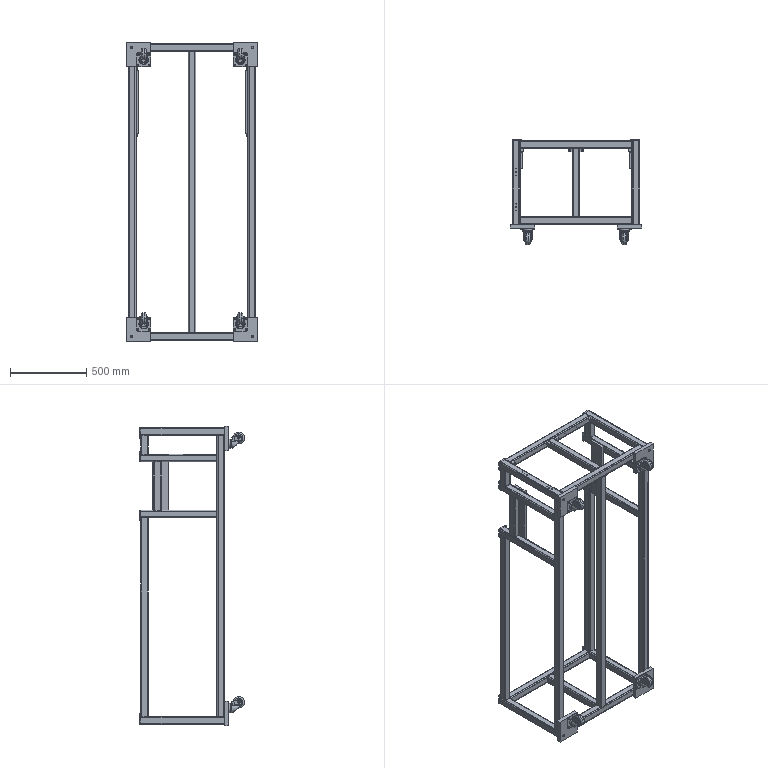Part | NX | features BREP 10 | 10 solids | 1291 faces | box 865 x 688.39 x 1967 mm | volume 11203517 mm3 | plane 667 | cylinder 516 | cone 44 | torus 32 | spline 32 | commonest cylinder face diameters 14 x136 10 x110 8 x80 6.8 x36 3.3 x34 9 x16